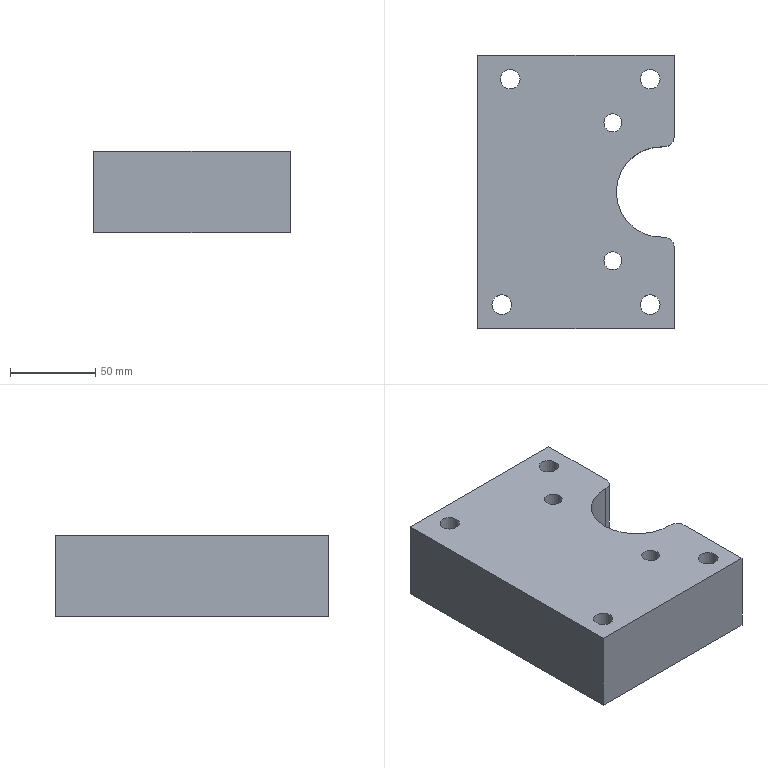Part | NX | features solid 2 | 1 solid | 46 faces | box 115 x 160 x 48 mm | volume 696890 mm3 | cylinder 23 | plane 21 | cone 2 | commonest cylinder face diameters 10 x8 11.509 x4 18.007 x4 8.5 x2 10.506 x2 12 x2
STEP:
#1=CARTESIAN_POINT('',(1221.76,10.689,65.));
#2=VERTEX_POINT('',#1);
#3=CARTESIAN_POINT('',(1277.226,25.551,65.));
#4=VERTEX_POINT('',#3);
#5=CARTESIAN_POINT('',(1303.344,32.549,65.));
#6=DIRECTION('',(0.9659,0.2588,0.));
#7=VECTOR('',#6,1000.);
#8=LINE('',#5,#7);
#9=EDGE_CURVE('',#2,#4,#8,.T.);
#10=ORIENTED_EDGE('',*,*,#9,.F.);
#11=CARTESIAN_POINT('',(1213.14,15.666,65.));
#12=VERTEX_POINT('',#11);
#13=CARTESIAN_POINT('',(1217.211,12.764,65.));
#14=DIRECTION('',(0.,0.,1.));
#15=DIRECTION('',(1.,0.,0.));
#16=AXIS2_PLACEMENT_3D('',#13,#14,#15);
#17=CIRCLE('',#16,5.);
#18=EDGE_CURVE('',#12,#2,#17,.T.);
#19=ORIENTED_EDGE('',*,*,#18,.F.);
#20=CARTESIAN_POINT('',(1207.724,35.876,65.));
#21=VERTEX_POINT('',#20);
#22=CARTESIAN_POINT('',(1203.025,53.415,65.));
#23=DIRECTION('',(0.2588,-0.9659,0.));
#24=VECTOR('',#23,1000.);
#25=LINE('',#22,#24);
#26=EDGE_CURVE('',#21,#12,#25,.T.);
#27=ORIENTED_EDGE('',*,*,#26,.F.);
#28=CARTESIAN_POINT('',(1212.702,44.496,65.));
#29=VERTEX_POINT('',#28);
#30=CARTESIAN_POINT('',(1209.8,40.425,65.));
#31=DIRECTION('',(0.,0.,1.));
#32=DIRECTION('',(1.,0.,0.));
#33=AXIS2_PLACEMENT_3D('',#30,#31,#32);
#34=CIRCLE('',#33,5.);
#35=EDGE_CURVE('',#29,#21,#34,.T.);
#36=ORIENTED_EDGE('',*,*,#35,.F.);
#37=CARTESIAN_POINT('',(1268.167,59.358,65.));
#38=VERTEX_POINT('',#37);
#39=CARTESIAN_POINT('',(1213.147,44.616,65.));
#40=DIRECTION('',(0.9659,0.2588,0.));
#41=VECTOR('',#40,1000.);
#42=LINE('',#39,#41);
#43=EDGE_CURVE('',#38,#29,#42,.F.);
#44=ORIENTED_EDGE('',*,*,#43,.F.);
#45=CARTESIAN_POINT('',(1276.788,54.381,65.));
#46=VERTEX_POINT('',#45);
#47=CARTESIAN_POINT('',(1272.716,57.283,65.));
#48=DIRECTION('',(0.,0.,1.));
#49=DIRECTION('',(1.,0.,0.));
#50=AXIS2_PLACEMENT_3D('',#47,#48,#49);
#51=CIRCLE('',#50,5.);
#52=EDGE_CURVE('',#46,#38,#51,.T.);
#53=ORIENTED_EDGE('',*,*,#52,.F.);
#54=CARTESIAN_POINT('',(1282.203,34.172,65.));
#55=VERTEX_POINT('',#54);
#56=CARTESIAN_POINT('',(1284.231,26.602,65.));
#57=DIRECTION('',(-0.2588,0.9659,0.));
#58=VECTOR('',#57,1000.);
#59=LINE('',#56,#58);
#60=EDGE_CURVE('',#55,#46,#59,.T.);
#61=ORIENTED_EDGE('',*,*,#60,.F.);
#62=CARTESIAN_POINT('',(1280.128,29.623,65.));
#63=DIRECTION('',(0.,0.,1.));
#64=DIRECTION('',(1.,0.,0.));
#65=AXIS2_PLACEMENT_3D('',#62,#63,#64);
#66=CIRCLE('',#65,5.);
#67=EDGE_CURVE('',#4,#55,#66,.T.);
#68=ORIENTED_EDGE('',*,*,#67,.F.);
#69=EDGE_LOOP('',(#10,#19,#27,#36,#44,#53,#61,#68));
#70=FACE_BOUND('',#69,.T.);
#71=CARTESIAN_POINT('',(1270.26,40.394,65.));
#72=VERTEX_POINT('',#71);
#73=CARTESIAN_POINT('',(1265.007,40.394,65.));
#74=DIRECTION('',(0.,0.,-1.));
#75=DIRECTION('',(1.,0.,0.));
#76=AXIS2_PLACEMENT_3D('',#73,#74,#75);
#77=CIRCLE('',#76,5.253);
#78=EDGE_CURVE('',#72,#72,#77,.T.);
#79=ORIENTED_EDGE('',*,*,#78,.F.);
#80=EDGE_LOOP('',(#79));
#81=FACE_BOUND('',#80,.T.);
#82=CARTESIAN_POINT('',(1243.403,-0.1294,65.));
#83=DIRECTION('',(0.,0.,1.));
#84=DIRECTION('',(1.,0.,0.));
#85=AXIS2_PLACEMENT_3D('',#82,#83,#84);
#86=PLANE('',#85);
#87=ADVANCED_FACE('',(#70,#81),#86,.F.);
#88=CARTESIAN_POINT('',(1212.702,-44.496,65.));
#89=VERTEX_POINT('',#88);
#90=CARTESIAN_POINT('',(1269.133,-59.617,65.));
#91=VERTEX_POINT('',#90);
#92=CARTESIAN_POINT('',(1213.147,-44.616,65.));
#93=DIRECTION('',(0.9659,-0.2588,0.));
#94=VECTOR('',#93,1000.);
#95=LINE('',#92,#94);
#96=EDGE_CURVE('',#89,#91,#95,.T.);
#97=ORIENTED_EDGE('',*,*,#96,.F.);
#98=CARTESIAN_POINT('',(1207.724,-35.876,65.));
#99=VERTEX_POINT('',#98);
#100=CARTESIAN_POINT('',(1209.8,-40.425,65.));
#101=DIRECTION('',(0.,0.,1.));
#102=DIRECTION('',(1.,0.,0.));
#103=AXIS2_PLACEMENT_3D('',#100,#101,#102);
#104=CIRCLE('',#103,5.);
#105=EDGE_CURVE('',#99,#89,#104,.T.);
#106=ORIENTED_EDGE('',*,*,#105,.F.);
#107=CARTESIAN_POINT('',(1213.14,-15.666,65.));
#108=VERTEX_POINT('',#107);
#109=CARTESIAN_POINT('',(1203.025,-53.415,65.));
#110=DIRECTION('',(0.2588,0.9659,0.));
#111=VECTOR('',#110,1000.);
#112=LINE('',#109,#111);
#113=EDGE_CURVE('',#108,#99,#112,.F.);
#114=ORIENTED_EDGE('',*,*,#113,.F.);
#115=CARTESIAN_POINT('',(1221.76,-10.689,65.));
#116=VERTEX_POINT('',#115);
#117=CARTESIAN_POINT('',(1217.211,-12.764,65.));
#118=DIRECTION('',(0.,0.,1.));
#119=DIRECTION('',(1.,0.,0.));
#120=AXIS2_PLACEMENT_3D('',#117,#118,#119);
#121=CIRCLE('',#120,5.);
#122=EDGE_CURVE('',#116,#108,#121,.T.);
#123=ORIENTED_EDGE('',*,*,#122,.F.);
#124=CARTESIAN_POINT('',(1278.192,-25.81,65.));
#125=VERTEX_POINT('',#124);
#126=CARTESIAN_POINT('',(1303.344,-32.549,65.));
#127=DIRECTION('',(0.9659,-0.2588,0.));
#128=VECTOR('',#127,1000.);
#129=LINE('',#126,#128);
#130=EDGE_CURVE('',#125,#116,#129,.F.);
#131=ORIENTED_EDGE('',*,*,#130,.F.);
#132=CARTESIAN_POINT('',(1283.169,-34.431,65.));
#133=VERTEX_POINT('',#132);
#134=CARTESIAN_POINT('',(1281.094,-29.882,65.));
#135=DIRECTION('',(0.,0.,1.));
#136=DIRECTION('',(1.,0.,0.));
#137=AXIS2_PLACEMENT_3D('',#134,#135,#136);
#138=CIRCLE('',#137,5.);
#139=EDGE_CURVE('',#133,#125,#138,.T.);
#140=ORIENTED_EDGE('',*,*,#139,.F.);
#141=CARTESIAN_POINT('',(1277.754,-54.64,65.));
#142=VERTEX_POINT('',#141);
#143=CARTESIAN_POINT('',(1223.832,-255.879,65.));
#144=DIRECTION('',(-0.2588,-0.9659,0.));
#145=VECTOR('',#144,1000.);
#146=LINE('',#143,#145);
#147=EDGE_CURVE('',#142,#133,#146,.F.);
#148=ORIENTED_EDGE('',*,*,#147,.F.);
#149=CARTESIAN_POINT('',(1273.682,-57.542,65.));
#150=DIRECTION('',(0.,0.,1.));
#151=DIRECTION('',(1.,0.,0.));
#152=AXIS2_PLACEMENT_3D('',#149,#150,#151);
#153=CIRCLE('',#152,5.);
#154=EDGE_CURVE('',#91,#142,#153,.T.);
#155=ORIENTED_EDGE('',*,*,#154,.F.);
#156=EDGE_LOOP('',(#97,#106,#114,#123,#131,#140,#148,#155));
#157=FACE_BOUND('',#156,.T.);
#158=CARTESIAN_POINT('',(1270.26,-40.394,65.));
#159=VERTEX_POINT('',#158);
#160=CARTESIAN_POINT('',(1265.007,-40.394,65.));
#161=DIRECTION('',(0.,0.,-1.));
#162=DIRECTION('',(1.,0.,0.));
#163=AXIS2_PLACEMENT_3D('',#160,#161,#162);
#164=CIRCLE('',#163,5.253);
#165=EDGE_CURVE('',#159,#159,#164,.T.);
#166=ORIENTED_EDGE('',*,*,#165,.F.);
#167=EDGE_LOOP('',(#166));
#168=FACE_BOUND('',#167,.T.);
#169=CARTESIAN_POINT('',(1243.403,-0.1294,65.));
#170=DIRECTION('',(0.,0.,1.));
#171=DIRECTION('',(1.,0.,0.));
#172=AXIS2_PLACEMENT_3D('',#169,#170,#171);
#173=PLANE('',#172);
#174=ADVANCED_FACE('',(#157,#168),#173,.F.);
#175=CARTESIAN_POINT('',(1239.153,64.871,50.));
#176=VERTEX_POINT('',#175);
#177=CARTESIAN_POINT('',(1243.403,64.871,50.));
#178=DIRECTION('',(0.,0.,-1.));
#179=DIRECTION('',(-1.,0.,0.));
#180=AXIS2_PLACEMENT_3D('',#177,#178,#179);
#181=CIRCLE('',#180,4.25);
#182=EDGE_CURVE('',#176,#176,#181,.T.);
#183=ORIENTED_EDGE('',*,*,#182,.F.);
#184=EDGE_LOOP('',(#183));
#185=FACE_BOUND('',#184,.T.);
#186=CARTESIAN_POINT('',(1239.153,-65.129,50.));
#187=VERTEX_POINT('',#186);
#188=CARTESIAN_POINT('',(1243.403,-65.129,50.));
#189=DIRECTION('',(0.,0.,-1.));
#190=DIRECTION('',(-1.,0.,0.));
#191=AXIS2_PLACEMENT_3D('',#188,#189,#190);
#192=CIRCLE('',#191,4.25);
#193=EDGE_CURVE('',#187,#187,#192,.T.);
#194=ORIENTED_EDGE('',*,*,#193,.F.);
#195=EDGE_LOOP('',(#194));
#196=FACE_BOUND('',#195,.T.);
#197=CARTESIAN_POINT('',(1269.133,-59.617,50.));
#198=VERTEX_POINT('',#197);
#199=CARTESIAN_POINT('',(1212.702,-44.496,50.));
#200=VERTEX_POINT('',#199);
#201=CARTESIAN_POINT('',(1121.617,-20.09,50.));
#202=DIRECTION('',(0.9659,-0.2588,0.));
#203=VECTOR('',#202,1000.);
#204=LINE('',#201,#203);
#205=EDGE_CURVE('',#198,#200,#204,.F.);
#206=ORIENTED_EDGE('',*,*,#205,.F.);
#207=CARTESIAN_POINT('',(1277.754,-54.64,50.));
#208=VERTEX_POINT('',#207);
#209=CARTESIAN_POINT('',(1273.682,-57.542,50.));
#210=DIRECTION('',(0.,0.,-1.));
#211=DIRECTION('',(-1.,0.,0.));
#212=AXIS2_PLACEMENT_3D('',#209,#210,#211);
#213=CIRCLE('',#212,5.);
#214=EDGE_CURVE('',#208,#198,#213,.T.);
#215=ORIENTED_EDGE('',*,*,#214,.F.);
#216=CARTESIAN_POINT('',(1283.169,-34.431,50.));
#217=VERTEX_POINT('',#216);
#218=CARTESIAN_POINT('',(1281.315,-41.349,50.));
#219=DIRECTION('',(-0.2588,-0.9659,0.));
#220=VECTOR('',#219,1000.);
#221=LINE('',#218,#220);
#222=EDGE_CURVE('',#217,#208,#221,.T.);
#223=ORIENTED_EDGE('',*,*,#222,.F.);
#224=CARTESIAN_POINT('',(1278.192,-25.81,50.));
#225=VERTEX_POINT('',#224);
#226=CARTESIAN_POINT('',(1281.094,-29.882,50.));
#227=DIRECTION('',(0.,0.,-1.));
#228=DIRECTION('',(-1.,0.,0.));
#229=AXIS2_PLACEMENT_3D('',#226,#227,#228);
#230=CIRCLE('',#229,5.);
#231=EDGE_CURVE('',#225,#217,#230,.T.);
#232=ORIENTED_EDGE('',*,*,#231,.F.);
#233=CARTESIAN_POINT('',(1221.76,-10.689,50.));
#234=VERTEX_POINT('',#233);
#235=CARTESIAN_POINT('',(1130.675,13.717,50.));
#236=DIRECTION('',(0.9659,-0.2588,0.));
#237=VECTOR('',#236,1000.);
#238=LINE('',#235,#237);
#239=EDGE_CURVE('',#234,#225,#238,.T.);
#240=ORIENTED_EDGE('',*,*,#239,.F.);
#241=CARTESIAN_POINT('',(1213.14,-15.666,50.));
#242=VERTEX_POINT('',#241);
#243=CARTESIAN_POINT('',(1217.211,-12.764,50.));
#244=DIRECTION('',(0.,0.,-1.));
#245=DIRECTION('',(-1.,0.,0.));
#246=AXIS2_PLACEMENT_3D('',#243,#244,#245);
#247=CIRCLE('',#246,5.);
#248=EDGE_CURVE('',#242,#234,#247,.T.);
#249=ORIENTED_EDGE('',*,*,#248,.F.);
#250=CARTESIAN_POINT('',(1207.724,-35.876,50.));
#251=VERTEX_POINT('',#250);
#252=CARTESIAN_POINT('',(1211.286,-22.584,50.));
#253=DIRECTION('',(0.2588,0.9659,0.));
#254=VECTOR('',#253,1000.);
#255=LINE('',#252,#254);
#256=EDGE_CURVE('',#251,#242,#255,.T.);
#257=ORIENTED_EDGE('',*,*,#256,.F.);
#258=CARTESIAN_POINT('',(1209.8,-40.425,50.));
#259=DIRECTION('',(0.,0.,-1.));
#260=DIRECTION('',(-1.,0.,0.));
#261=AXIS2_PLACEMENT_3D('',#258,#259,#260);
#262=CIRCLE('',#261,5.);
#263=EDGE_CURVE('',#200,#251,#262,.T.);
#264=ORIENTED_EDGE('',*,*,#263,.F.);
#265=EDGE_LOOP('',(#206,#215,#223,#232,#240,#249,#257,#264));
#266=FACE_BOUND('',#265,.T.);
#267=CARTESIAN_POINT('',(1277.226,25.551,50.));
#268=VERTEX_POINT('',#267);
#269=CARTESIAN_POINT('',(1221.76,10.689,50.));
#270=VERTEX_POINT('',#269);
#271=CARTESIAN_POINT('',(1130.675,-13.717,50.));
#272=DIRECTION('',(0.9659,0.2588,0.));
#273=VECTOR('',#272,1000.);
#274=LINE('',#271,#273);
#275=EDGE_CURVE('',#268,#270,#274,.F.);
#276=ORIENTED_EDGE('',*,*,#275,.F.);
#277=CARTESIAN_POINT('',(1282.203,34.172,50.));
#278=VERTEX_POINT('',#277);
#279=CARTESIAN_POINT('',(1280.128,29.623,50.));
#280=DIRECTION('',(0.,0.,-1.));
#281=DIRECTION('',(-1.,0.,0.));
#282=AXIS2_PLACEMENT_3D('',#279,#280,#281);
#283=CIRCLE('',#282,5.);
#284=EDGE_CURVE('',#278,#268,#283,.T.);
#285=ORIENTED_EDGE('',*,*,#284,.F.);
#286=CARTESIAN_POINT('',(1276.788,54.381,50.));
#287=VERTEX_POINT('',#286);
#288=CARTESIAN_POINT('',(1280.35,41.09,50.));
#289=DIRECTION('',(-0.2588,0.9659,0.));
#290=VECTOR('',#289,1000.);
#291=LINE('',#288,#290);
#292=EDGE_CURVE('',#287,#278,#291,.F.);
#293=ORIENTED_EDGE('',*,*,#292,.F.);
#294=CARTESIAN_POINT('',(1268.167,59.358,50.));
#295=VERTEX_POINT('',#294);
#296=CARTESIAN_POINT('',(1272.716,57.283,50.));
#297=DIRECTION('',(0.,0.,-1.));
#298=DIRECTION('',(-1.,0.,0.));
#299=AXIS2_PLACEMENT_3D('',#296,#297,#298);
#300=CIRCLE('',#299,5.);
#301=EDGE_CURVE('',#295,#287,#300,.T.);
#302=ORIENTED_EDGE('',*,*,#301,.F.);
#303=CARTESIAN_POINT('',(1212.702,44.496,50.));
#304=VERTEX_POINT('',#303);
#305=CARTESIAN_POINT('',(1121.617,20.09,50.));
#306=DIRECTION('',(0.9659,0.2588,0.));
#307=VECTOR('',#306,1000.);
#308=LINE('',#305,#307);
#309=EDGE_CURVE('',#304,#295,#308,.T.);
#310=ORIENTED_EDGE('',*,*,#309,.F.);
#311=CARTESIAN_POINT('',(1207.724,35.876,50.));
#312=VERTEX_POINT('',#311);
#313=CARTESIAN_POINT('',(1209.8,40.425,50.));
#314=DIRECTION('',(0.,0.,-1.));
#315=DIRECTION('',(-1.,0.,0.));
#316=AXIS2_PLACEMENT_3D('',#313,#314,#315);
#317=CIRCLE('',#316,5.);
#318=EDGE_CURVE('',#312,#304,#317,.T.);
#319=ORIENTED_EDGE('',*,*,#318,.F.);
#320=CARTESIAN_POINT('',(1213.14,15.666,50.));
#321=VERTEX_POINT('',#320);
#322=CARTESIAN_POINT('',(1211.286,22.584,50.));
#323=DIRECTION('',(0.2588,-0.9659,0.));
#324=VECTOR('',#323,1000.);
#325=LINE('',#322,#324);
#326=EDGE_CURVE('',#321,#312,#325,.F.);
#327=ORIENTED_EDGE('',*,*,#326,.F.);
#328=CARTESIAN_POINT('',(1217.211,12.764,50.));
#329=DIRECTION('',(0.,0.,-1.));
#330=DIRECTION('',(-1.,0.,0.));
#331=AXIS2_PLACEMENT_3D('',#328,#329,#330);
#332=CIRCLE('',#331,5.);
#333=EDGE_CURVE('',#270,#321,#332,.T.);
#334=ORIENTED_EDGE('',*,*,#333,.F.);
#335=EDGE_LOOP('',(#276,#285,#293,#302,#310,#319,#327,#334));
#336=FACE_BOUND('',#335,.T.);
#337=CARTESIAN_POINT('',(1208.906,-66.129,50.));
#338=VERTEX_POINT('',#337);
#339=CARTESIAN_POINT('',(1199.903,-66.129,50.));
#340=DIRECTION('',(0.,0.,1.));
#341=DIRECTION('',(1.,0.,0.));
#342=AXIS2_PLACEMENT_3D('',#339,#340,#341);
#343=CIRCLE('',#342,9.004);
#344=EDGE_CURVE('',#338,#338,#343,.T.);
#345=ORIENTED_EDGE('',*,*,#344,.T.);
#346=EDGE_LOOP('',(#345));
#347=FACE_BOUND('',#346,.T.);
#348=CARTESIAN_POINT('',(1213.906,65.871,50.));
#349=VERTEX_POINT('',#348);
#350=CARTESIAN_POINT('',(1204.903,65.871,50.));
#351=DIRECTION('',(0.,0.,1.));
#352=DIRECTION('',(1.,0.,0.));
#353=AXIS2_PLACEMENT_3D('',#350,#351,#352);
#354=CIRCLE('',#353,9.004);
#355=EDGE_CURVE('',#349,#349,#354,.T.);
#356=ORIENTED_EDGE('',*,*,#355,.T.);
#357=EDGE_LOOP('',(#356));
#358=FACE_BOUND('',#357,.T.);
#359=CARTESIAN_POINT('',(1300.903,79.871,50.));
#360=VERTEX_POINT('',#359);
#361=CARTESIAN_POINT('',(1300.903,32.315,50.));
#362=VERTEX_POINT('',#361);
#363=CARTESIAN_POINT('',(1300.903,0.,50.));
#364=DIRECTION('',(0.,-1.,0.));
#365=VECTOR('',#364,1000.);
#366=LINE('',#363,#365);
#367=EDGE_CURVE('',#360,#362,#366,.T.);
#368=ORIENTED_EDGE('',*,*,#367,.T.);
#369=CARTESIAN_POINT('',(1294.644,26.32,50.));
#370=VERTEX_POINT('',#369);
#371=CARTESIAN_POINT('',(1294.903,32.315,50.));
#372=DIRECTION('',(0.,0.,-1.));
#373=DIRECTION('',(-1.,0.,0.));
#374=AXIS2_PLACEMENT_3D('',#371,#372,#373);
#375=CIRCLE('',#374,6.);
#376=EDGE_CURVE('',#362,#370,#375,.T.);
#377=ORIENTED_EDGE('',*,*,#376,.T.);
#378=CARTESIAN_POINT('',(1294.644,-26.63,50.));
#379=VERTEX_POINT('',#378);
#380=CARTESIAN_POINT('',(1293.5,-0.1549,50.));
#381=DIRECTION('',(0.,0.,-1.));
#382=DIRECTION('',(-1.,0.,0.));
#383=AXIS2_PLACEMENT_3D('',#380,#381,#382);
#384=CIRCLE('',#383,26.5);
#385=EDGE_CURVE('',#370,#379,#384,.F.);
#386=ORIENTED_EDGE('',*,*,#385,.T.);
#387=CARTESIAN_POINT('',(1300.903,-32.625,50.));
#388=VERTEX_POINT('',#387);
#389=CARTESIAN_POINT('',(1294.903,-32.625,50.));
#390=DIRECTION('',(0.,0.,-1.));
#391=DIRECTION('',(-1.,0.,0.));
#392=AXIS2_PLACEMENT_3D('',#389,#390,#391);
#393=CIRCLE('',#392,6.);
#394=EDGE_CURVE('',#379,#388,#393,.T.);
#395=ORIENTED_EDGE('',*,*,#394,.T.);
#396=CARTESIAN_POINT('',(1300.903,-80.129,50.));
#397=VERTEX_POINT('',#396);
#398=CARTESIAN_POINT('',(1300.903,0.,50.));
#399=DIRECTION('',(0.,-1.,0.));
#400=VECTOR('',#399,1000.);
#401=LINE('',#398,#400);
#402=EDGE_CURVE('',#388,#397,#401,.T.);
#403=ORIENTED_EDGE('',*,*,#402,.T.);
#404=CARTESIAN_POINT('',(1185.903,-80.129,50.));
#405=VERTEX_POINT('',#404);
#406=CARTESIAN_POINT('',(1127.,-80.129,50.));
#407=DIRECTION('',(-1.,0.,0.));
#408=VECTOR('',#407,1000.);
#409=LINE('',#406,#408);
#410=EDGE_CURVE('',#397,#405,#409,.T.);
#411=ORIENTED_EDGE('',*,*,#410,.T.);
#412=CARTESIAN_POINT('',(1185.903,79.871,50.));
#413=VERTEX_POINT('',#412);
#414=CARTESIAN_POINT('',(1185.903,-0.1294,50.));
#415=DIRECTION('',(0.,-1.,0.));
#416=VECTOR('',#415,1000.);
#417=LINE('',#414,#416);
#418=EDGE_CURVE('',#413,#405,#417,.T.);
#419=ORIENTED_EDGE('',*,*,#418,.F.);
#420=CARTESIAN_POINT('',(1127.,79.871,50.));
#421=DIRECTION('',(1.,0.,0.));
#422=VECTOR('',#421,1000.);
#423=LINE('',#420,#422);
#424=EDGE_CURVE('',#413,#360,#423,.T.);
#425=ORIENTED_EDGE('',*,*,#424,.T.);
#426=EDGE_LOOP('',(#368,#377,#386,#395,#403,#411,#419,#425));
#427=FACE_BOUND('',#426,.T.);
#428=CARTESIAN_POINT('',(1295.906,65.871,50.));
#429=VERTEX_POINT('',#428);
#430=CARTESIAN_POINT('',(1286.903,65.871,50.));
#431=DIRECTION('',(0.,0.,1.));
#432=DIRECTION('',(1.,0.,0.));
#433=AXIS2_PLACEMENT_3D('',#430,#431,#432);
#434=CIRCLE('',#433,9.004);
#435=EDGE_CURVE('',#429,#429,#434,.T.);
#436=ORIENTED_EDGE('',*,*,#435,.T.);
#437=EDGE_LOOP('',(#436));
#438=FACE_BOUND('',#437,.T.);
#439=CARTESIAN_POINT('',(1295.906,-66.129,50.));
#440=VERTEX_POINT('',#439);
#441=CARTESIAN_POINT('',(1286.903,-66.129,50.));
#442=DIRECTION('',(0.,0.,1.));
#443=DIRECTION('',(1.,0.,0.));
#444=AXIS2_PLACEMENT_3D('',#441,#442,#443);
#445=CIRCLE('',#444,9.004);
#446=EDGE_CURVE('',#440,#440,#445,.T.);
#447=ORIENTED_EDGE('',*,*,#446,.T.);
#448=EDGE_LOOP('',(#447));
#449=FACE_BOUND('',#448,.T.);
#450=CARTESIAN_POINT('',(1127.,0.,50.));
#451=DIRECTION('',(0.,0.,-1.));
#452=DIRECTION('',(-1.,0.,0.));
#453=AXIS2_PLACEMENT_3D('',#450,#451,#452);
#454=PLANE('',#453);
#455=ADVANCED_FACE('',(#185,#196,#266,#336,#347,#358,#427,#438,#449),#454,.T.);
#456=CARTESIAN_POINT('',(1300.903,32.315,98.));
#457=VERTEX_POINT('',#456);
#458=CARTESIAN_POINT('',(1300.903,79.871,98.));
#459=VERTEX_POINT('',#458);
#460=CARTESIAN_POINT('',(1300.903,0.,98.));
#461=DIRECTION('',(0.,1.,0.));
#462=VECTOR('',#461,1000.);
#463=LINE('',#460,#462);
#464=EDGE_CURVE('',#457,#459,#463,.T.);
#465=ORIENTED_EDGE('',*,*,#464,.F.);
#466=CARTESIAN_POINT('',(1300.903,32.315,69.));
#467=DIRECTION('',(0.,0.,1.));
#468=VECTOR('',#467,1000.);
#469=LINE('',#466,#468);
#470=EDGE_CURVE('',#457,#362,#469,.F.);
#471=ORIENTED_EDGE('',*,*,#470,.T.);
#472=ORIENTED_EDGE('',*,*,#367,.F.);
#473=CARTESIAN_POINT('',(1300.903,79.871,69.));
#474=DIRECTION('',(0.,0.,1.));
#475=VECTOR('',#474,1000.);
#476=LINE('',#473,#475);
#477=EDGE_CURVE('',#360,#459,#476,.T.);
#478=ORIENTED_EDGE('',*,*,#477,.T.);
#479=EDGE_LOOP('',(#465,#471,#472,#478));
#480=FACE_BOUND('',#479,.T.);
#481=CARTESIAN_POINT('',(1300.903,-0.1294,69.));
#482=DIRECTION('',(1.,0.,0.));
#483=DIRECTION('',(0.,0.,-1.));
#484=AXIS2_PLACEMENT_3D('',#481,#482,#483);
#485=PLANE('',#484);
#486=ADVANCED_FACE('',(#480),#485,.T.);
#487=ORIENTED_EDGE('',*,*,#402,.F.);
#488=CARTESIAN_POINT('',(1300.903,-32.625,98.));
#489=VERTEX_POINT('',#488);
#490=CARTESIAN_POINT('',(1300.903,-32.625,69.));
#491=DIRECTION('',(0.,0.,1.));
#492=VECTOR('',#491,1000.);
#493=LINE('',#490,#492);
#494=EDGE_CURVE('',#388,#489,#493,.T.);
#495=ORIENTED_EDGE('',*,*,#494,.T.);
#496=CARTESIAN_POINT('',(1300.903,-80.129,98.));
#497=VERTEX_POINT('',#496);
#498=CARTESIAN_POINT('',(1300.903,0.,98.));
#499=DIRECTION('',(0.,1.,0.));
#500=VECTOR('',#499,1000.);
#501=LINE('',#498,#500);
#502=EDGE_CURVE('',#497,#489,#501,.T.);
#503=ORIENTED_EDGE('',*,*,#502,.F.);
#504=CARTESIAN_POINT('',(1300.903,-80.129,69.));
#505=DIRECTION('',(0.,0.,-1.));
#506=VECTOR('',#505,1000.);
#507=LINE('',#504,#506);
#508=EDGE_CURVE('',#497,#397,#507,.T.);
#509=ORIENTED_EDGE('',*,*,#508,.T.);
#510=EDGE_LOOP('',(#487,#495,#503,#509));
#511=FACE_BOUND('',#510,.T.);
#512=CARTESIAN_POINT('',(1300.903,-0.1294,69.));
#513=DIRECTION('',(1.,0.,0.));
#514=DIRECTION('',(0.,0.,-1.));
#515=AXIS2_PLACEMENT_3D('',#512,#513,#514);
#516=PLANE('',#515);
#517=ADVANCED_FACE('',(#511),#516,.T.);
#518=CARTESIAN_POINT('',(1270.26,40.394,98.));
#519=VERTEX_POINT('',#518);
#520=CARTESIAN_POINT('',(1265.007,40.394,98.));
#521=DIRECTION('',(0.,0.,1.));
#522=DIRECTION('',(1.,0.,0.));
#523=AXIS2_PLACEMENT_3D('',#520,#521,#522);
#524=CIRCLE('',#523,5.253);
#525=EDGE_CURVE('',#519,#519,#524,.T.);
#526=ORIENTED_EDGE('',*,*,#525,.F.);
#527=EDGE_LOOP('',(#526));
#528=FACE_BOUND('',#527,.T.);
#529=CARTESIAN_POINT('',(1270.26,-40.394,98.));
#530=VERTEX_POINT('',#529);
#531=CARTESIAN_POINT('',(1265.007,-40.394,98.));
#532=DIRECTION('',(0.,0.,1.));
#533=DIRECTION('',(1.,0.,0.));
#534=AXIS2_PLACEMENT_3D('',#531,#532,#533);
#535=CIRCLE('',#534,5.253);
#536=EDGE_CURVE('',#530,#530,#535,.T.);
#537=ORIENTED_EDGE('',*,*,#536,.F.);
#538=EDGE_LOOP('',(#537));
#539=FACE_BOUND('',#538,.T.);
#540=CARTESIAN_POINT('',(1292.657,-66.129,98.));
#541=VERTEX_POINT('',#540);
#542=CARTESIAN_POINT('',(1286.903,-66.129,98.));
#543=DIRECTION('',(0.,0.,1.));
#544=DIRECTION('',(1.,0.,0.));
#545=AXIS2_PLACEMENT_3D('',#542,#543,#544);
#546=CIRCLE('',#545,5.755);
#547=EDGE_CURVE('',#541,#541,#546,.T.);
#548=ORIENTED_EDGE('',*,*,#547,.F.);
#549=EDGE_LOOP('',(#548));
#550=FACE_BOUND('',#549,.T.);
#551=CARTESIAN_POINT('',(1205.657,-66.129,98.));
#552=VERTEX_POINT('',#551);
#553=CARTESIAN_POINT('',(1199.903,-66.129,98.));
#554=DIRECTION('',(0.,0.,1.));
#555=DIRECTION('',(1.,0.,0.));
#556=AXIS2_PLACEMENT_3D('',#553,#554,#555);
#557=CIRCLE('',#556,5.755);
#558=EDGE_CURVE('',#552,#552,#557,.T.);
#559=ORIENTED_EDGE('',*,*,#558,.F.);
#560=EDGE_LOOP('',(#559));
#561=FACE_BOUND('',#560,.T.);
#562=CARTESIAN_POINT('',(1292.657,65.871,98.));
#563=VERTEX_POINT('',#562);
#564=CARTESIAN_POINT('',(1286.903,65.871,98.));
#565=DIRECTION('',(0.,0.,1.));
#566=DIRECTION('',(1.,0.,0.));
#567=AXIS2_PLACEMENT_3D('',#564,#565,#566);
#568=CIRCLE('',#567,5.755);
#569=EDGE_CURVE('',#563,#563,#568,.T.);
#570=ORIENTED_EDGE('',*,*,#569,.F.);
#571=EDGE_LOOP('',(#570));
#572=FACE_BOUND('',#571,.T.);
#573=CARTESIAN_POINT('',(1210.657,65.871,98.));
#574=VERTEX_POINT('',#573);
#575=CARTESIAN_POINT('',(1204.903,65.871,98.));
#576=DIRECTION('',(0.,0.,1.));
#577=DIRECTION('',(1.,0.,0.));
#578=AXIS2_PLACEMENT_3D('',#575,#576,#577);
#579=CIRCLE('',#578,5.755);
#580=EDGE_CURVE('',#574,#574,#579,.T.);
#581=ORIENTED_EDGE('',*,*,#580,.F.);
#582=EDGE_LOOP('',(#581));
#583=FACE_BOUND('',#582,.T.);
#584=CARTESIAN_POINT('',(1294.644,-26.63,98.));
#585=VERTEX_POINT('',#584);
#586=CARTESIAN_POINT('',(1294.644,26.32,98.));
#587=VERTEX_POINT('',#586);
#588=CARTESIAN_POINT('',(1293.5,-0.1549,98.));
#589=DIRECTION('',(0.,0.,1.));
#590=DIRECTION('',(1.,0.,0.));
#591=AXIS2_PLACEMENT_3D('',#588,#589,#590);
#592=CIRCLE('',#591,26.5);
#593=EDGE_CURVE('',#585,#587,#592,.F.);
#594=ORIENTED_EDGE('',*,*,#593,.T.);
#595=CARTESIAN_POINT('',(1294.903,32.315,98.));
#596=DIRECTION('',(0.,0.,1.));
#597=DIRECTION('',(1.,0.,0.));
#598=AXIS2_PLACEMENT_3D('',#595,#596,#597);
#599=CIRCLE('',#598,6.);
#600=EDGE_CURVE('',#587,#457,#599,.T.);
#601=ORIENTED_EDGE('',*,*,#600,.T.);
#602=ORIENTED_EDGE('',*,*,#464,.T.);
#603=CARTESIAN_POINT('',(1185.903,79.871,98.));
#604=VERTEX_POINT('',#603);
#605=CARTESIAN_POINT('',(835.5,79.871,98.));
#606=DIRECTION('',(-1.,0.,0.));
#607=VECTOR('',#606,1000.);
#608=LINE('',#605,#607);
#609=EDGE_CURVE('',#459,#604,#608,.T.);
#610=ORIENTED_EDGE('',*,*,#609,.T.);
#611=CARTESIAN_POINT('',(1185.903,-80.129,98.));
#612=VERTEX_POINT('',#611);
#613=CARTESIAN_POINT('',(1185.903,-0.1294,98.));
#614=DIRECTION('',(0.,1.,0.));
#615=VECTOR('',#614,1000.);
#616=LINE('',#613,#615);
#617=EDGE_CURVE('',#612,#604,#616,.T.);
#618=ORIENTED_EDGE('',*,*,#617,.F.);
#619=CARTESIAN_POINT('',(835.5,-80.129,98.));
#620=DIRECTION('',(1.,0.,0.));
#621=VECTOR('',#620,1000.);
#622=LINE('',#619,#621);
#623=EDGE_CURVE('',#612,#497,#622,.T.);
#624=ORIENTED_EDGE('',*,*,#623,.T.);
#625=ORIENTED_EDGE('',*,*,#502,.T.);
#626=CARTESIAN_POINT('',(1294.903,-32.625,98.));
#627=DIRECTION('',(0.,0.,1.));
#628=DIRECTION('',(1.,0.,0.));
#629=AXIS2_PLACEMENT_3D('',#626,#627,#628);
#630=CIRCLE('',#629,6.);
#631=EDGE_CURVE('',#489,#585,#630,.T.);
#632=ORIENTED_EDGE('',*,*,#631,.T.);
#633=EDGE_LOOP('',(#594,#601,#602,#610,#618,#624,#625,#632));
#634=FACE_BOUND('',#633,.T.);
#635=CARTESIAN_POINT('',(835.5,0.,98.));
#636=DIRECTION('',(0.,0.,1.));
#637=DIRECTION('',(1.,0.,0.));
#638=AXIS2_PLACEMENT_3D('',#635,#636,#637);
#639=PLANE('',#638);
#640=ADVANCED_FACE('',(#528,#539,#550,#561,#572,#583,#634),#639,.T.);
#641=ORIENTED_EDGE('',*,*,#477,.F.);
#642=ORIENTED_EDGE('',*,*,#424,.F.);
#643=CARTESIAN_POINT('',(1185.903,79.871,-33.4));
#644=DIRECTION('',(0.,0.,-1.));
#645=VECTOR('',#644,1000.);
#646=LINE('',#643,#645);
#647=EDGE_CURVE('',#604,#413,#646,.T.);
#648=ORIENTED_EDGE('',*,*,#647,.F.);
#649=ORIENTED_EDGE('',*,*,#609,.F.);
#650=EDGE_LOOP('',(#641,#642,#648,#649));
#651=FACE_BOUND('',#650,.T.);
#652=CARTESIAN_POINT('',(1295.903,79.871,50.));
#653=DIRECTION('',(0.,1.,0.));
#654=DIRECTION('',(0.,0.,1.));
#655=AXIS2_PLACEMENT_3D('',#652,#653,#654);
#656=PLANE('',#655);
#657=ADVANCED_FACE('',(#651),#656,.T.);
#658=ORIENTED_EDGE('',*,*,#617,.T.);
#659=ORIENTED_EDGE('',*,*,#647,.T.);
#660=ORIENTED_EDGE('',*,*,#418,.T.);
#661=CARTESIAN_POINT('',(1185.903,-80.129,-33.4));
#662=DIRECTION('',(0.,0.,1.));
#663=VECTOR('',#662,1000.);
#664=LINE('',#661,#663);
#665=EDGE_CURVE('',#405,#612,#664,.T.);
#666=ORIENTED_EDGE('',*,*,#665,.T.);
#667=EDGE_LOOP('',(#658,#659,#660,#666));
#668=FACE_BOUND('',#667,.T.);
#669=CARTESIAN_POINT('',(1185.903,-0.1294,-33.4));
#670=DIRECTION('',(-1.,0.,0.));
#671=DIRECTION('',(0.,0.,1.));
#672=AXIS2_PLACEMENT_3D('',#669,#670,#671);
#673=PLANE('',#672);
#674=ADVANCED_FACE('',(#668),#673,.T.);
#675=ORIENTED_EDGE('',*,*,#508,.F.);
#676=ORIENTED_EDGE('',*,*,#623,.F.);
#677=ORIENTED_EDGE('',*,*,#665,.F.);
#678=ORIENTED_EDGE('',*,*,#410,.F.);
#679=EDGE_LOOP('',(#675,#676,#677,#678));
#680=FACE_BOUND('',#679,.T.);
#681=CARTESIAN_POINT('',(1295.903,-80.129,50.));
#682=DIRECTION('',(0.,-1.,0.));
#683=DIRECTION('',(0.,0.,-1.));
#684=AXIS2_PLACEMENT_3D('',#681,#682,#683);
#685=PLANE('',#684);
#686=ADVANCED_FACE('',(#680),#685,.T.);
#687=ORIENTED_EDGE('',*,*,#385,.F.);
#688=CARTESIAN_POINT('',(1294.644,26.32,50.));
#689=DIRECTION('',(0.,0.,1.));
#690=VECTOR('',#689,1000.);
#691=LINE('',#688,#690);
#692=EDGE_CURVE('',#370,#587,#691,.T.);
#693=ORIENTED_EDGE('',*,*,#692,.T.);
#694=ORIENTED_EDGE('',*,*,#593,.F.);
#695=CARTESIAN_POINT('',(1294.644,-26.63,98.));
#696=DIRECTION('',(0.,0.,1.));
#697=VECTOR('',#696,1000.);
#698=LINE('',#695,#697);
#699=EDGE_CURVE('',#585,#379,#698,.F.);
#700=ORIENTED_EDGE('',*,*,#699,.T.);
#701=EDGE_LOOP('',(#687,#693,#694,#700));
#702=FACE_BOUND('',#701,.T.);
#703=CARTESIAN_POINT('',(1293.5,-0.1549,114.));
#704=DIRECTION('',(0.,0.,1.));
#705=DIRECTION('',(1.,0.,0.));
#706=AXIS2_PLACEMENT_3D('',#703,#704,#705);
#707=CYLINDRICAL_SURFACE('',#706,26.5);
#708=ADVANCED_FACE('',(#702),#707,.F.);
#709=ORIENTED_EDGE('',*,*,#600,.F.);
#710=ORIENTED_EDGE('',*,*,#692,.F.);
#711=ORIENTED_EDGE('',*,*,#376,.F.);
#712=ORIENTED_EDGE('',*,*,#470,.F.);
#713=EDGE_LOOP('',(#709,#710,#711,#712));
#714=FACE_BOUND('',#713,.T.);
#715=CARTESIAN_POINT('',(1294.903,32.315,114.));
#716=DIRECTION('',(0.,0.,1.));
#717=DIRECTION('',(1.,0.,0.));
#718=AXIS2_PLACEMENT_3D('',#715,#716,#717);
#719=CYLINDRICAL_SURFACE('',#718,6.);
#720=ADVANCED_FACE('',(#714),#719,.T.);
#721=ORIENTED_EDGE('',*,*,#394,.F.);
#722=ORIENTED_EDGE('',*,*,#699,.F.);
#723=ORIENTED_EDGE('',*,*,#631,.F.);
#724=ORIENTED_EDGE('',*,*,#494,.F.);
#725=EDGE_LOOP('',(#721,#722,#723,#724));
#726=FACE_BOUND('',#725,.T.);
#727=CARTESIAN_POINT('',(1294.903,-32.625,114.));
#728=DIRECTION('',(0.,0.,1.));
#729=DIRECTION('',(1.,0.,0.));
#730=AXIS2_PLACEMENT_3D('',#727,#728,#729);
#731=CYLINDRICAL_SURFACE('',#730,6.);
#732=ADVANCED_FACE('',(#726),#731,.T.);
#733=ORIENTED_EDGE('',*,*,#580,.T.);
#734=EDGE_LOOP('',(#733));
#735=FACE_BOUND('',#734,.T.);
#736=CARTESIAN_POINT('',(1210.657,65.871,63.));
#737=VERTEX_POINT('',#736);
#738=CARTESIAN_POINT('',(1204.903,65.871,63.));
#739=DIRECTION('',(0.,0.,1.));
#740=DIRECTION('',(1.,0.,0.));
#741=AXIS2_PLACEMENT_3D('',#738,#739,#740);
#742=CIRCLE('',#741,5.755);
#743=EDGE_CURVE('',#737,#737,#742,.T.);
#744=ORIENTED_EDGE('',*,*,#743,.F.);
#745=EDGE_LOOP('',(#744));
#746=FACE_BOUND('',#745,.T.);
#747=CARTESIAN_POINT('',(1204.903,65.871,45.));
#748=DIRECTION('',(0.,0.,1.));
#749=DIRECTION('',(1.,0.,0.));
#750=AXIS2_PLACEMENT_3D('',#747,#748,#749);
#751=CYLINDRICAL_SURFACE('',#750,5.755);
#752=ADVANCED_FACE('',(#735,#746),#751,.F.);
#753=ORIENTED_EDGE('',*,*,#743,.T.);
#754=EDGE_LOOP('',(#753));
#755=FACE_BOUND('',#754,.T.);
#756=CARTESIAN_POINT('',(1213.906,65.871,63.));
#757=VERTEX_POINT('',#756);
#758=CARTESIAN_POINT('',(1204.903,65.871,63.));
#759=DIRECTION('',(0.,0.,-1.));
#760=DIRECTION('',(1.,0.,0.));
#761=AXIS2_PLACEMENT_3D('',#758,#759,#760);
#762=CIRCLE('',#761,9.004);
#763=EDGE_CURVE('',#757,#757,#762,.F.);
#764=ORIENTED_EDGE('',*,*,#763,.F.);
#765=EDGE_LOOP('',(#764));
#766=FACE_BOUND('',#765,.T.);
#767=CARTESIAN_POINT('',(1204.903,65.871,63.));
#768=DIRECTION('',(0.,0.,1.));
#769=DIRECTION('',(1.,0.,0.));
#770=AXIS2_PLACEMENT_3D('',#767,#768,#769);
#771=PLANE('',#770);
#772=ADVANCED_FACE('',(#755,#766),#771,.F.);
#773=ORIENTED_EDGE('',*,*,#763,.T.);
#774=EDGE_LOOP('',(#773));
#775=FACE_BOUND('',#774,.T.);
#776=ORIENTED_EDGE('',*,*,#355,.F.);
#777=EDGE_LOOP('',(#776));
#778=FACE_BOUND('',#777,.T.);
#779=CARTESIAN_POINT('',(1204.903,65.871,50.));
#780=DIRECTION('',(0.,0.,1.));
#781=DIRECTION('',(1.,0.,0.));
#782=AXIS2_PLACEMENT_3D('',#779,#780,#781);
#783=CYLINDRICAL_SURFACE('',#782,9.004);
#784=ADVANCED_FACE('',(#775,#778),#783,.F.);
#785=ORIENTED_EDGE('',*,*,#569,.T.);
#786=EDGE_LOOP('',(#785));
#787=FACE_BOUND('',#786,.T.);
#788=CARTESIAN_POINT('',(1292.657,65.871,63.));
#789=VERTEX_POINT('',#788);
#790=CARTESIAN_POINT('',(1286.903,65.871,63.));
#791=DIRECTION('',(0.,0.,1.));
#792=DIRECTION('',(1.,0.,0.));
#793=AXIS2_PLACEMENT_3D('',#790,#791,#792);
#794=CIRCLE('',#793,5.755);
#795=EDGE_CURVE('',#789,#789,#794,.T.);
#796=ORIENTED_EDGE('',*,*,#795,.F.);
#797=EDGE_LOOP('',(#796));
#798=FACE_BOUND('',#797,.T.);
#799=CARTESIAN_POINT('',(1286.903,65.871,45.));
#800=DIRECTION('',(0.,0.,1.));
#801=DIRECTION('',(1.,0.,0.));
#802=AXIS2_PLACEMENT_3D('',#799,#800,#801);
#803=CYLINDRICAL_SURFACE('',#802,5.755);
#804=ADVANCED_FACE('',(#787,#798),#803,.F.);
#805=ORIENTED_EDGE('',*,*,#795,.T.);
#806=EDGE_LOOP('',(#805));
#807=FACE_BOUND('',#806,.T.);
#808=CARTESIAN_POINT('',(1295.906,65.871,63.));
#809=VERTEX_POINT('',#808);
#810=CARTESIAN_POINT('',(1286.903,65.871,63.));
#811=DIRECTION('',(0.,0.,-1.));
#812=DIRECTION('',(1.,0.,0.));
#813=AXIS2_PLACEMENT_3D('',#810,#811,#812);
#814=CIRCLE('',#813,9.004);
#815=EDGE_CURVE('',#809,#809,#814,.F.);
#816=ORIENTED_EDGE('',*,*,#815,.F.);
#817=EDGE_LOOP('',(#816));
#818=FACE_BOUND('',#817,.T.);
#819=CARTESIAN_POINT('',(1286.903,65.871,63.));
#820=DIRECTION('',(0.,0.,1.));
#821=DIRECTION('',(1.,0.,0.));
#822=AXIS2_PLACEMENT_3D('',#819,#820,#821);
#823=PLANE('',#822);
#824=ADVANCED_FACE('',(#807,#818),#823,.F.);
#825=ORIENTED_EDGE('',*,*,#815,.T.);
#826=EDGE_LOOP('',(#825));
#827=FACE_BOUND('',#826,.T.);
#828=ORIENTED_EDGE('',*,*,#435,.F.);
#829=EDGE_LOOP('',(#828));
#830=FACE_BOUND('',#829,.T.);
#831=CARTESIAN_POINT('',(1286.903,65.871,50.));
#832=DIRECTION('',(0.,0.,1.));
#833=DIRECTION('',(1.,0.,0.));
#834=AXIS2_PLACEMENT_3D('',#831,#832,#833);
#835=CYLINDRICAL_SURFACE('',#834,9.004);
#836=ADVANCED_FACE('',(#827,#830),#835,.F.);
#837=ORIENTED_EDGE('',*,*,#558,.T.);
#838=EDGE_LOOP('',(#837));
#839=FACE_BOUND('',#838,.T.);
#840=CARTESIAN_POINT('',(1205.657,-66.129,63.));
#841=VERTEX_POINT('',#840);
#842=CARTESIAN_POINT('',(1199.903,-66.129,63.));
#843=DIRECTION('',(0.,0.,1.));
#844=DIRECTION('',(1.,0.,0.));
#845=AXIS2_PLACEMENT_3D('',#842,#843,#844);
#846=CIRCLE('',#845,5.755);
#847=EDGE_CURVE('',#841,#841,#846,.T.);
#848=ORIENTED_EDGE('',*,*,#847,.F.);
#849=EDGE_LOOP('',(#848));
#850=FACE_BOUND('',#849,.T.);
#851=CARTESIAN_POINT('',(1199.903,-66.129,45.));
#852=DIRECTION('',(0.,0.,1.));
#853=DIRECTION('',(1.,0.,0.));
#854=AXIS2_PLACEMENT_3D('',#851,#852,#853);
#855=CYLINDRICAL_SURFACE('',#854,5.755);
#856=ADVANCED_FACE('',(#839,#850),#855,.F.);
#857=ORIENTED_EDGE('',*,*,#847,.T.);
#858=EDGE_LOOP('',(#857));
#859=FACE_BOUND('',#858,.T.);
#860=CARTESIAN_POINT('',(1208.906,-66.129,63.));
#861=VERTEX_POINT('',#860);
#862=CARTESIAN_POINT('',(1199.903,-66.129,63.));
#863=DIRECTION('',(0.,0.,-1.));
#864=DIRECTION('',(1.,0.,0.));
#865=AXIS2_PLACEMENT_3D('',#862,#863,#864);
#866=CIRCLE('',#865,9.004);
#867=EDGE_CURVE('',#861,#861,#866,.F.);
#868=ORIENTED_EDGE('',*,*,#867,.F.);
#869=EDGE_LOOP('',(#868));
#870=FACE_BOUND('',#869,.T.);
#871=CARTESIAN_POINT('',(1199.903,-66.129,63.));
#872=DIRECTION('',(0.,0.,1.));
#873=DIRECTION('',(1.,0.,0.));
#874=AXIS2_PLACEMENT_3D('',#871,#872,#873);
#875=PLANE('',#874);
#876=ADVANCED_FACE('',(#859,#870),#875,.F.);
#877=ORIENTED_EDGE('',*,*,#867,.T.);
#878=EDGE_LOOP('',(#877));
#879=FACE_BOUND('',#878,.T.);
#880=ORIENTED_EDGE('',*,*,#344,.F.);
#881=EDGE_LOOP('',(#880));
#882=FACE_BOUND('',#881,.T.);
#883=CARTESIAN_POINT('',(1199.903,-66.129,50.));
#884=DIRECTION('',(0.,0.,1.));
#885=DIRECTION('',(1.,0.,0.));
#886=AXIS2_PLACEMENT_3D('',#883,#884,#885);
#887=CYLINDRICAL_SURFACE('',#886,9.004);
#888=ADVANCED_FACE('',(#879,#882),#887,.F.);
#889=ORIENTED_EDGE('',*,*,#547,.T.);
#890=EDGE_LOOP('',(#889));
#891=FACE_BOUND('',#890,.T.);
#892=CARTESIAN_POINT('',(1292.657,-66.129,63.));
#893=VERTEX_POINT('',#892);
#894=CARTESIAN_POINT('',(1286.903,-66.129,63.));
#895=DIRECTION('',(0.,0.,1.));
#896=DIRECTION('',(1.,0.,0.));
#897=AXIS2_PLACEMENT_3D('',#894,#895,#896);
#898=CIRCLE('',#897,5.755);
#899=EDGE_CURVE('',#893,#893,#898,.T.);
#900=ORIENTED_EDGE('',*,*,#899,.F.);
#901=EDGE_LOOP('',(#900));
#902=FACE_BOUND('',#901,.T.);
#903=CARTESIAN_POINT('',(1286.903,-66.129,45.));
#904=DIRECTION('',(0.,0.,1.));
#905=DIRECTION('',(1.,0.,0.));
#906=AXIS2_PLACEMENT_3D('',#903,#904,#905);
#907=CYLINDRICAL_SURFACE('',#906,5.755);
#908=ADVANCED_FACE('',(#891,#902),#907,.F.);
#909=ORIENTED_EDGE('',*,*,#899,.T.);
#910=EDGE_LOOP('',(#909));
#911=FACE_BOUND('',#910,.T.);
#912=CARTESIAN_POINT('',(1295.906,-66.129,63.));
#913=VERTEX_POINT('',#912);
#914=CARTESIAN_POINT('',(1286.903,-66.129,63.));
#915=DIRECTION('',(0.,0.,-1.));
#916=DIRECTION('',(1.,0.,0.));
#917=AXIS2_PLACEMENT_3D('',#914,#915,#916);
#918=CIRCLE('',#917,9.004);
#919=EDGE_CURVE('',#913,#913,#918,.F.);
#920=ORIENTED_EDGE('',*,*,#919,.F.);
#921=EDGE_LOOP('',(#920));
#922=FACE_BOUND('',#921,.T.);
#923=CARTESIAN_POINT('',(1286.903,-66.129,63.));
#924=DIRECTION('',(0.,0.,1.));
#925=DIRECTION('',(1.,0.,0.));
#926=AXIS2_PLACEMENT_3D('',#923,#924,#925);
#927=PLANE('',#926);
#928=ADVANCED_FACE('',(#911,#922),#927,.F.);
#929=ORIENTED_EDGE('',*,*,#919,.T.);
#930=EDGE_LOOP('',(#929));
#931=FACE_BOUND('',#930,.T.);
#932=ORIENTED_EDGE('',*,*,#446,.F.);
#933=EDGE_LOOP('',(#932));
#934=FACE_BOUND('',#933,.T.);
#935=CARTESIAN_POINT('',(1286.903,-66.129,50.));
#936=DIRECTION('',(0.,0.,1.));
#937=DIRECTION('',(1.,0.,0.));
#938=AXIS2_PLACEMENT_3D('',#935,#936,#937);
#939=CYLINDRICAL_SURFACE('',#938,9.004);
#940=ADVANCED_FACE('',(#931,#934),#939,.F.);
#941=ORIENTED_EDGE('',*,*,#275,.T.);
#942=CARTESIAN_POINT('',(1221.76,10.689,103.));
#943=DIRECTION('',(0.,0.,-1.));
#944=VECTOR('',#943,1000.);
#945=LINE('',#942,#944);
#946=EDGE_CURVE('',#270,#2,#945,.F.);
#947=ORIENTED_EDGE('',*,*,#946,.T.);
#948=ORIENTED_EDGE('',*,*,#9,.T.);
#949=CARTESIAN_POINT('',(1277.226,25.551,103.));
#950=DIRECTION('',(0.,0.,-1.));
#951=VECTOR('',#950,1000.);
#952=LINE('',#949,#951);
#953=EDGE_CURVE('',#268,#4,#952,.F.);
#954=ORIENTED_EDGE('',*,*,#953,.F.);
#955=EDGE_LOOP('',(#941,#947,#948,#954));
#956=FACE_BOUND('',#955,.T.);
#957=CARTESIAN_POINT('',(1303.344,32.549,103.));
#958=DIRECTION('',(-0.2588,0.9659,0.));
#959=DIRECTION('',(-0.9659,-0.2588,0.));
#960=AXIS2_PLACEMENT_3D('',#957,#958,#959);
#961=PLANE('',#960);
#962=ADVANCED_FACE('',(#956),#961,.T.);
#963=ORIENTED_EDGE('',*,*,#333,.T.);
#964=CARTESIAN_POINT('',(1213.14,15.666,103.));
#965=DIRECTION('',(0.,0.,-1.));
#966=VECTOR('',#965,1000.);
#967=LINE('',#964,#966);
#968=EDGE_CURVE('',#321,#12,#967,.F.);
#969=ORIENTED_EDGE('',*,*,#968,.T.);
#970=ORIENTED_EDGE('',*,*,#18,.T.);
#971=ORIENTED_EDGE('',*,*,#946,.F.);
#972=EDGE_LOOP('',(#963,#969,#970,#971));
#973=FACE_BOUND('',#972,.T.);
#974=CARTESIAN_POINT('',(1217.211,12.764,103.));
#975=DIRECTION('',(0.,0.,-1.));
#976=DIRECTION('',(-1.,0.,0.));
#977=AXIS2_PLACEMENT_3D('',#974,#975,#976);
#978=CYLINDRICAL_SURFACE('',#977,5.);
#979=ADVANCED_FACE('',(#973),#978,.F.);
#980=ORIENTED_EDGE('',*,*,#326,.T.);
#981=CARTESIAN_POINT('',(1207.724,35.876,103.));
#982=DIRECTION('',(0.,0.,-1.));
#983=VECTOR('',#982,1000.);
#984=LINE('',#981,#983);
#985=EDGE_CURVE('',#312,#21,#984,.F.);
#986=ORIENTED_EDGE('',*,*,#985,.T.);
#987=ORIENTED_EDGE('',*,*,#26,.T.);
#988=ORIENTED_EDGE('',*,*,#968,.F.);
#989=EDGE_LOOP('',(#980,#986,#987,#988));
#990=FACE_BOUND('',#989,.T.);
#991=CARTESIAN_POINT('',(1203.025,53.415,103.));
#992=DIRECTION('',(0.9659,0.2588,0.));
#993=DIRECTION('',(-0.2588,0.9659,0.));
#994=AXIS2_PLACEMENT_3D('',#991,#992,#993);
#995=PLANE('',#994);
#996=ADVANCED_FACE('',(#990),#995,.T.);
#997=ORIENTED_EDGE('',*,*,#318,.T.);
#998=CARTESIAN_POINT('',(1212.702,44.496,103.));
#999=DIRECTION('',(0.,0.,-1.));
#1000=VECTOR('',#999,1000.);
#1001=LINE('',#998,#1000);
#1002=EDGE_CURVE('',#304,#29,#1001,.F.);
#1003=ORIENTED_EDGE('',*,*,#1002,.T.);
#1004=ORIENTED_EDGE('',*,*,#35,.T.);
#1005=ORIENTED_EDGE('',*,*,#985,.F.);
#1006=EDGE_LOOP('',(#997,#1003,#1004,#1005));
#1007=FACE_BOUND('',#1006,.T.);
#1008=CARTESIAN_POINT('',(1209.8,40.425,103.));
#1009=DIRECTION('',(0.,0.,-1.));
#1010=DIRECTION('',(-1.,0.,0.));
#1011=AXIS2_PLACEMENT_3D('',#1008,#1009,#1010);
#1012=CYLINDRICAL_SURFACE('',#1011,5.);
#1013=ADVANCED_FACE('',(#1007),#1012,.F.);
#1014=ORIENTED_EDGE('',*,*,#309,.T.);
#1015=CARTESIAN_POINT('',(1268.167,59.358,103.));
#1016=DIRECTION('',(0.,0.,-1.));
#1017=VECTOR('',#1016,1000.);
#1018=LINE('',#1015,#1017);
#1019=EDGE_CURVE('',#295,#38,#1018,.F.);
#1020=ORIENTED_EDGE('',*,*,#1019,.T.);
#1021=ORIENTED_EDGE('',*,*,#43,.T.);
#1022=ORIENTED_EDGE('',*,*,#1002,.F.);
#1023=EDGE_LOOP('',(#1014,#1020,#1021,#1022));
#1024=FACE_BOUND('',#1023,.T.);
#1025=CARTESIAN_POINT('',(1213.147,44.616,103.));
#1026=DIRECTION('',(-0.2588,0.9659,0.));
#1027=DIRECTION('',(-0.9659,-0.2588,0.));
#1028=AXIS2_PLACEMENT_3D('',#1025,#1026,#1027);
#1029=PLANE('',#1028);
#1030=ADVANCED_FACE('',(#1024),#1029,.F.);
#1031=ORIENTED_EDGE('',*,*,#301,.T.);
#1032=CARTESIAN_POINT('',(1276.788,54.381,103.));
#1033=DIRECTION('',(0.,0.,-1.));
#1034=VECTOR('',#1033,1000.);
#1035=LINE('',#1032,#1034);
#1036=EDGE_CURVE('',#287,#46,#1035,.F.);
#1037=ORIENTED_EDGE('',*,*,#1036,.T.);
#1038=ORIENTED_EDGE('',*,*,#52,.T.);
#1039=ORIENTED_EDGE('',*,*,#1019,.F.);
#1040=EDGE_LOOP('',(#1031,#1037,#1038,#1039));
#1041=FACE_BOUND('',#1040,.T.);
#1042=CARTESIAN_POINT('',(1272.716,57.283,103.));
#1043=DIRECTION('',(0.,0.,-1.));
#1044=DIRECTION('',(-1.,0.,0.));
#1045=AXIS2_PLACEMENT_3D('',#1042,#1043,#1044);
#1046=CYLINDRICAL_SURFACE('',#1045,5.);
#1047=ADVANCED_FACE('',(#1041),#1046,.F.);
#1048=ORIENTED_EDGE('',*,*,#292,.T.);
#1049=CARTESIAN_POINT('',(1282.203,34.172,103.));
#1050=DIRECTION('',(0.,0.,-1.));
#1051=VECTOR('',#1050,1000.);
#1052=LINE('',#1049,#1051);
#1053=EDGE_CURVE('',#278,#55,#1052,.F.);
#1054=ORIENTED_EDGE('',*,*,#1053,.T.);
#1055=ORIENTED_EDGE('',*,*,#60,.T.);
#1056=ORIENTED_EDGE('',*,*,#1036,.F.);
#1057=EDGE_LOOP('',(#1048,#1054,#1055,#1056));
#1058=FACE_BOUND('',#1057,.T.);
#1059=CARTESIAN_POINT('',(1284.231,26.602,103.));
#1060=DIRECTION('',(-0.9659,-0.2588,0.));
#1061=DIRECTION('',(0.2588,-0.9659,0.));
#1062=AXIS2_PLACEMENT_3D('',#1059,#1060,#1061);
#1063=PLANE('',#1062);
#1064=ADVANCED_FACE('',(#1058),#1063,.T.);
#1065=ORIENTED_EDGE('',*,*,#284,.T.);
#1066=ORIENTED_EDGE('',*,*,#953,.T.);
#1067=ORIENTED_EDGE('',*,*,#67,.T.);
#1068=ORIENTED_EDGE('',*,*,#1053,.F.);
#1069=EDGE_LOOP('',(#1065,#1066,#1067,#1068));
#1070=FACE_BOUND('',#1069,.T.);
#1071=CARTESIAN_POINT('',(1280.128,29.623,103.));
#1072=DIRECTION('',(0.,0.,-1.));
#1073=DIRECTION('',(-1.,0.,0.));
#1074=AXIS2_PLACEMENT_3D('',#1071,#1072,#1073);
#1075=CYLINDRICAL_SURFACE('',#1074,5.);
#1076=ADVANCED_FACE('',(#1070),#1075,.F.);
#1077=ORIENTED_EDGE('',*,*,#205,.T.);
#1078=CARTESIAN_POINT('',(1212.702,-44.496,103.));
#1079=DIRECTION('',(0.,0.,-1.));
#1080=VECTOR('',#1079,1000.);
#1081=LINE('',#1078,#1080);
#1082=EDGE_CURVE('',#200,#89,#1081,.F.);
#1083=ORIENTED_EDGE('',*,*,#1082,.T.);
#1084=ORIENTED_EDGE('',*,*,#96,.T.);
#1085=CARTESIAN_POINT('',(1269.133,-59.617,103.));
#1086=DIRECTION('',(0.,0.,-1.));
#1087=VECTOR('',#1086,1000.);
#1088=LINE('',#1085,#1087);
#1089=EDGE_CURVE('',#198,#91,#1088,.F.);
#1090=ORIENTED_EDGE('',*,*,#1089,.F.);
#1091=EDGE_LOOP('',(#1077,#1083,#1084,#1090));
#1092=FACE_BOUND('',#1091,.T.);
#1093=CARTESIAN_POINT('',(1213.147,-44.616,103.));
#1094=DIRECTION('',(0.2588,0.9659,0.));
#1095=DIRECTION('',(-0.9659,0.2588,0.));
#1096=AXIS2_PLACEMENT_3D('',#1093,#1094,#1095);
#1097=PLANE('',#1096);
#1098=ADVANCED_FACE('',(#1092),#1097,.T.);
#1099=ORIENTED_EDGE('',*,*,#263,.T.);
#1100=CARTESIAN_POINT('',(1207.724,-35.876,103.));
#1101=DIRECTION('',(0.,0.,-1.));
#1102=VECTOR('',#1101,1000.);
#1103=LINE('',#1100,#1102);
#1104=EDGE_CURVE('',#251,#99,#1103,.F.);
#1105=ORIENTED_EDGE('',*,*,#1104,.T.);
#1106=ORIENTED_EDGE('',*,*,#105,.T.);
#1107=ORIENTED_EDGE('',*,*,#1082,.F.);
#1108=EDGE_LOOP('',(#1099,#1105,#1106,#1107));
#1109=FACE_BOUND('',#1108,.T.);
#1110=CARTESIAN_POINT('',(1209.8,-40.425,103.));
#1111=DIRECTION('',(0.,0.,-1.));
#1112=DIRECTION('',(-1.,0.,0.));
#1113=AXIS2_PLACEMENT_3D('',#1110,#1111,#1112);
#1114=CYLINDRICAL_SURFACE('',#1113,5.);
#1115=ADVANCED_FACE('',(#1109),#1114,.F.);
#1116=ORIENTED_EDGE('',*,*,#256,.T.);
#1117=CARTESIAN_POINT('',(1213.14,-15.666,103.));
#1118=DIRECTION('',(0.,0.,-1.));
#1119=VECTOR('',#1118,1000.);
#1120=LINE('',#1117,#1119);
#1121=EDGE_CURVE('',#242,#108,#1120,.F.);
#1122=ORIENTED_EDGE('',*,*,#1121,.T.);
#1123=ORIENTED_EDGE('',*,*,#113,.T.);
#1124=ORIENTED_EDGE('',*,*,#1104,.F.);
#1125=EDGE_LOOP('',(#1116,#1122,#1123,#1124));
#1126=FACE_BOUND('',#1125,.T.);
#1127=CARTESIAN_POINT('',(1203.025,-53.415,103.));
#1128=DIRECTION('',(-0.9659,0.2588,0.));
#1129=DIRECTION('',(-0.2588,-0.9659,0.));
#1130=AXIS2_PLACEMENT_3D('',#1127,#1128,#1129);
#1131=PLANE('',#1130);
#1132=ADVANCED_FACE('',(#1126),#1131,.F.);
#1133=ORIENTED_EDGE('',*,*,#248,.T.);
#1134=CARTESIAN_POINT('',(1221.76,-10.689,103.));
#1135=DIRECTION('',(0.,0.,-1.));
#1136=VECTOR('',#1135,1000.);
#1137=LINE('',#1134,#1136);
#1138=EDGE_CURVE('',#234,#116,#1137,.F.);
#1139=ORIENTED_EDGE('',*,*,#1138,.T.);
#1140=ORIENTED_EDGE('',*,*,#122,.T.);
#1141=ORIENTED_EDGE('',*,*,#1121,.F.);
#1142=EDGE_LOOP('',(#1133,#1139,#1140,#1141));
#1143=FACE_BOUND('',#1142,.T.);
#1144=CARTESIAN_POINT('',(1217.211,-12.764,103.));
#1145=DIRECTION('',(0.,0.,-1.));
#1146=DIRECTION('',(-1.,0.,0.));
#1147=AXIS2_PLACEMENT_3D('',#1144,#1145,#1146);
#1148=CYLINDRICAL_SURFACE('',#1147,5.);
#1149=ADVANCED_FACE('',(#1143),#1148,.F.);
#1150=ORIENTED_EDGE('',*,*,#239,.T.);
#1151=CARTESIAN_POINT('',(1278.192,-25.81,103.));
#1152=DIRECTION('',(0.,0.,-1.));
#1153=VECTOR('',#1152,1000.);
#1154=LINE('',#1151,#1153);
#1155=EDGE_CURVE('',#225,#125,#1154,.F.);
#1156=ORIENTED_EDGE('',*,*,#1155,.T.);
#1157=ORIENTED_EDGE('',*,*,#130,.T.);
#1158=ORIENTED_EDGE('',*,*,#1138,.F.);
#1159=EDGE_LOOP('',(#1150,#1156,#1157,#1158));
#1160=FACE_BOUND('',#1159,.T.);
#1161=CARTESIAN_POINT('',(1303.344,-32.549,103.));
#1162=DIRECTION('',(0.2588,0.9659,0.));
#1163=DIRECTION('',(-0.9659,0.2588,0.));
#1164=AXIS2_PLACEMENT_3D('',#1161,#1162,#1163);
#1165=PLANE('',#1164);
#1166=ADVANCED_FACE('',(#1160),#1165,.F.);
#1167=ORIENTED_EDGE('',*,*,#231,.T.);
#1168=CARTESIAN_POINT('',(1283.169,-34.431,103.));
#1169=DIRECTION('',(0.,0.,-1.));
#1170=VECTOR('',#1169,1000.);
#1171=LINE('',#1168,#1170);
#1172=EDGE_CURVE('',#217,#133,#1171,.F.);
#1173=ORIENTED_EDGE('',*,*,#1172,.T.);
#1174=ORIENTED_EDGE('',*,*,#139,.T.);
#1175=ORIENTED_EDGE('',*,*,#1155,.F.);
#1176=EDGE_LOOP('',(#1167,#1173,#1174,#1175));
#1177=FACE_BOUND('',#1176,.T.);
#1178=CARTESIAN_POINT('',(1281.094,-29.882,103.));
#1179=DIRECTION('',(0.,0.,-1.));
#1180=DIRECTION('',(-1.,0.,0.));
#1181=AXIS2_PLACEMENT_3D('',#1178,#1179,#1180);
#1182=CYLINDRICAL_SURFACE('',#1181,5.);
#1183=ADVANCED_FACE('',(#1177),#1182,.F.);
#1184=ORIENTED_EDGE('',*,*,#222,.T.);
#1185=CARTESIAN_POINT('',(1277.754,-54.64,103.));
#1186=DIRECTION('',(0.,0.,-1.));
#1187=VECTOR('',#1186,1000.);
#1188=LINE('',#1185,#1187);
#1189=EDGE_CURVE('',#208,#142,#1188,.F.);
#1190=ORIENTED_EDGE('',*,*,#1189,.T.);
#1191=ORIENTED_EDGE('',*,*,#147,.T.);
#1192=ORIENTED_EDGE('',*,*,#1172,.F.);
#1193=EDGE_LOOP('',(#1184,#1190,#1191,#1192));
#1194=FACE_BOUND('',#1193,.T.);
#1195=CARTESIAN_POINT('',(1223.832,-255.879,103.));
#1196=DIRECTION('',(0.9659,-0.2588,0.));
#1197=DIRECTION('',(0.2588,0.9659,0.));
#1198=AXIS2_PLACEMENT_3D('',#1195,#1196,#1197);
#1199=PLANE('',#1198);
#1200=ADVANCED_FACE('',(#1194),#1199,.F.);
#1201=ORIENTED_EDGE('',*,*,#214,.T.);
#1202=ORIENTED_EDGE('',*,*,#1089,.T.);
#1203=ORIENTED_EDGE('',*,*,#154,.T.);
#1204=ORIENTED_EDGE('',*,*,#1189,.F.);
#1205=EDGE_LOOP('',(#1201,#1202,#1203,#1204));
#1206=FACE_BOUND('',#1205,.T.);
#1207=CARTESIAN_POINT('',(1273.682,-57.542,103.));
#1208=DIRECTION('',(0.,0.,-1.));
#1209=DIRECTION('',(-1.,0.,0.));
#1210=AXIS2_PLACEMENT_3D('',#1207,#1208,#1209);
#1211=CYLINDRICAL_SURFACE('',#1210,5.);
#1212=ADVANCED_FACE('',(#1206),#1211,.F.);
#1213=CARTESIAN_POINT('',(1247.653,-65.129,70.));
#1214=VERTEX_POINT('',#1213);
#1215=CARTESIAN_POINT('',(1243.403,-65.129,70.));
#1216=DIRECTION('',(0.,0.,-1.));
#1217=DIRECTION('',(1.,0.,0.));
#1218=AXIS2_PLACEMENT_3D('',#1215,#1216,#1217);
#1219=CIRCLE('',#1218,4.25);
#1220=EDGE_CURVE('',#1214,#1214,#1219,.F.);
#1221=ORIENTED_EDGE('',*,*,#1220,.F.);
#1222=EDGE_LOOP('',(#1221));
#1223=FACE_BOUND('',#1222,.T.);
#1224=CARTESIAN_POINT('',(1243.403,-65.129,72.554));
#1225=VERTEX_POINT('',#1224);
#1226=VERTEX_LOOP('',#1225);
#1227=FACE_BOUND('',#1226,.T.);
#1228=CARTESIAN_POINT('',(1243.403,-65.129,70.));
#1229=DIRECTION('',(0.,0.,-1.));
#1230=DIRECTION('',(-1.,0.,0.));
#1231=AXIS2_PLACEMENT_3D('',#1228,#1229,#1230);
#1232=CONICAL_SURFACE('',#1231,4.25,1.03);
#1233=ADVANCED_FACE('',(#1223,#1227),#1232,.F.);
#1234=ORIENTED_EDGE('',*,*,#193,.T.);
#1235=EDGE_LOOP('',(#1234));
#1236=FACE_BOUND('',#1235,.T.);
#1237=ORIENTED_EDGE('',*,*,#1220,.T.);
#1238=EDGE_LOOP('',(#1237));
#1239=FACE_BOUND('',#1238,.T.);
#1240=CARTESIAN_POINT('',(1243.403,-65.129,50.));
#1241=DIRECTION('',(0.,0.,1.));
#1242=DIRECTION('',(1.,0.,0.));
#1243=AXIS2_PLACEMENT_3D('',#1240,#1241,#1242);
#1244=CYLINDRICAL_SURFACE('',#1243,4.25);
#1245=ADVANCED_FACE('',(#1236,#1239),#1244,.F.);
#1246=CARTESIAN_POINT('',(1247.653,64.871,70.));
#1247=VERTEX_POINT('',#1246);
#1248=CARTESIAN_POINT('',(1243.403,64.871,70.));
#1249=DIRECTION('',(0.,0.,1.));
#1250=DIRECTION('',(1.,0.,0.));
#1251=AXIS2_PLACEMENT_3D('',#1248,#1249,#1250);
#1252=CIRCLE('',#1251,4.25);
#1253=EDGE_CURVE('',#1247,#1247,#1252,.F.);
#1254=ORIENTED_EDGE('',*,*,#1253,.T.);
#1255=EDGE_LOOP('',(#1254));
#1256=FACE_BOUND('',#1255,.T.);
#1257=CARTESIAN_POINT('',(1243.403,64.871,72.554));
#1258=VERTEX_POINT('',#1257);
#1259=VERTEX_LOOP('',#1258);
#1260=FACE_BOUND('',#1259,.T.);
#1261=CARTESIAN_POINT('',(1243.403,64.871,70.));
#1262=DIRECTION('',(0.,0.,-1.));
#1263=DIRECTION('',(-1.,0.,0.));
#1264=AXIS2_PLACEMENT_3D('',#1261,#1262,#1263);
#1265=CONICAL_SURFACE('',#1264,4.25,1.03);
#1266=ADVANCED_FACE('',(#1256,#1260),#1265,.F.);
#1267=ORIENTED_EDGE('',*,*,#182,.T.);
#1268=EDGE_LOOP('',(#1267));
#1269=FACE_BOUND('',#1268,.T.);
#1270=ORIENTED_EDGE('',*,*,#1253,.F.);
#1271=EDGE_LOOP('',(#1270));
#1272=FACE_BOUND('',#1271,.T.);
#1273=CARTESIAN_POINT('',(1243.403,64.871,50.));
#1274=DIRECTION('',(0.,0.,1.));
#1275=DIRECTION('',(1.,0.,0.));
#1276=AXIS2_PLACEMENT_3D('',#1273,#1274,#1275);
#1277=CYLINDRICAL_SURFACE('',#1276,4.25);
#1278=ADVANCED_FACE('',(#1269,#1272),#1277,.F.);
#1279=ORIENTED_EDGE('',*,*,#536,.T.);
#1280=EDGE_LOOP('',(#1279));
#1281=FACE_BOUND('',#1280,.T.);
#1282=ORIENTED_EDGE('',*,*,#165,.T.);
#1283=EDGE_LOOP('',(#1282));
#1284=FACE_BOUND('',#1283,.T.);
#1285=CARTESIAN_POINT('',(1265.007,-40.394,65.));
#1286=DIRECTION('',(0.,0.,1.));
#1287=DIRECTION('',(1.,0.,0.));
#1288=AXIS2_PLACEMENT_3D('',#1285,#1286,#1287);
#1289=CYLINDRICAL_SURFACE('',#1288,5.253);
#1290=ADVANCED_FACE('',(#1281,#1284),#1289,.F.);
#1291=ORIENTED_EDGE('',*,*,#525,.T.);
#1292=EDGE_LOOP('',(#1291));
#1293=FACE_BOUND('',#1292,.T.);
#1294=ORIENTED_EDGE('',*,*,#78,.T.);
#1295=EDGE_LOOP('',(#1294));
#1296=FACE_BOUND('',#1295,.T.);
#1297=CARTESIAN_POINT('',(1265.007,40.394,65.));
#1298=DIRECTION('',(0.,0.,1.));
#1299=DIRECTION('',(1.,0.,0.));
#1300=AXIS2_PLACEMENT_3D('',#1297,#1298,#1299);
#1301=CYLINDRICAL_SURFACE('',#1300,5.253);
#1302=ADVANCED_FACE('',(#1293,#1296),#1301,.F.);
#1303=CLOSED_SHELL('',(#87,#174,#455,#486,#517,#640,#657,#674,#686,#708,#720,#732,#752,#772,#784,#804,#824,#836,#856,#876,#888,#908,#928,#940,#962,#979,#996,#1013,#1030,#1047,#1064,#1076,#1098,#1115,#1132,#1149,#1166,#1183,#1200,#1212,#1233,#1245,#1266,#1278,#1290,#1302));
#1304=MANIFOLD_SOLID_BREP('',#1303);
#1305=(LENGTH_UNIT()NAMED_UNIT(*)SI_UNIT(.MILLI.,.METRE.));
#1306=UNCERTAINTY_MEASURE_WITH_UNIT(LENGTH_MEASURE(0.00001),#1305,'','');
#1307=(NAMED_UNIT(*)PLANE_ANGLE_UNIT()SI_UNIT($,.RADIAN.));
#1308=(NAMED_UNIT(*)SI_UNIT($,.STERADIAN.)SOLID_ANGLE_UNIT());
#1309=(GEOMETRIC_REPRESENTATION_CONTEXT(3)GLOBAL_UNCERTAINTY_ASSIGNED_CONTEXT((#1306))GLOBAL_UNIT_ASSIGNED_CONTEXT((#1305,#1307,#1308))REPRESENTATION_CONTEXT('',''));
#1310=ADVANCED_BREP_SHAPE_REPRESENTATION('',(#1304),#1309);